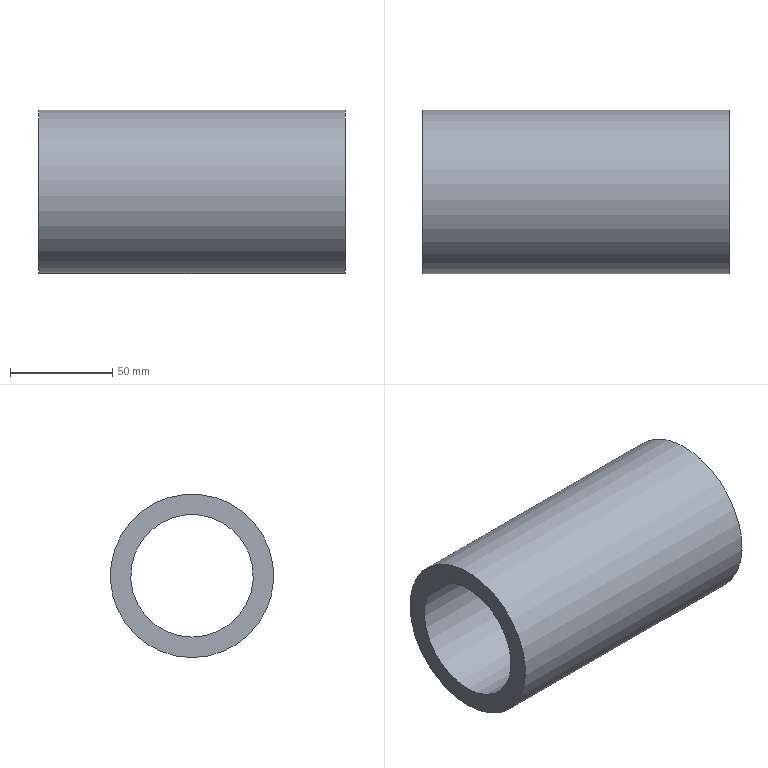Part | STEP file | solid 210 | 1 solid | 4 faces | box 150 x 80 x 80 mm | volume 329867 mm3 | plane 2 | cylinder 2 | commonest cylinder face diameters 60 x1 80 x1